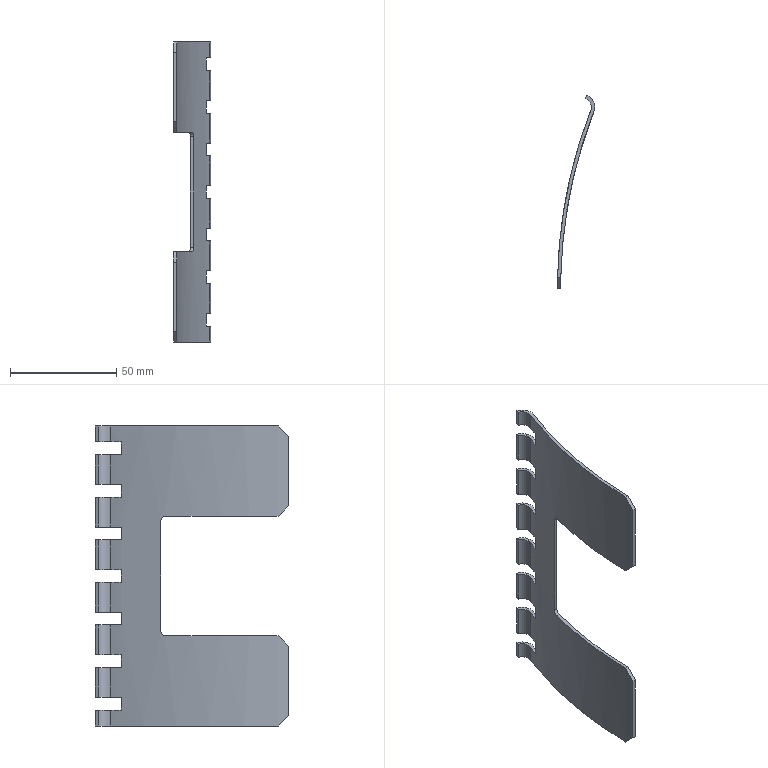Part | SolidWorks | features ICE 2, Chamfer 1, Extrusion 1, Fillet 1 | 1 solid | 60 faces | box 17.458 x 90.837 x 141 mm | volume 13768 mm3 | plane 32 | cylinder 28 | commonest cylinder face diameters 9 x8 12 x8 471.6 x8 4 x2 459.6 x1 462.6 x1